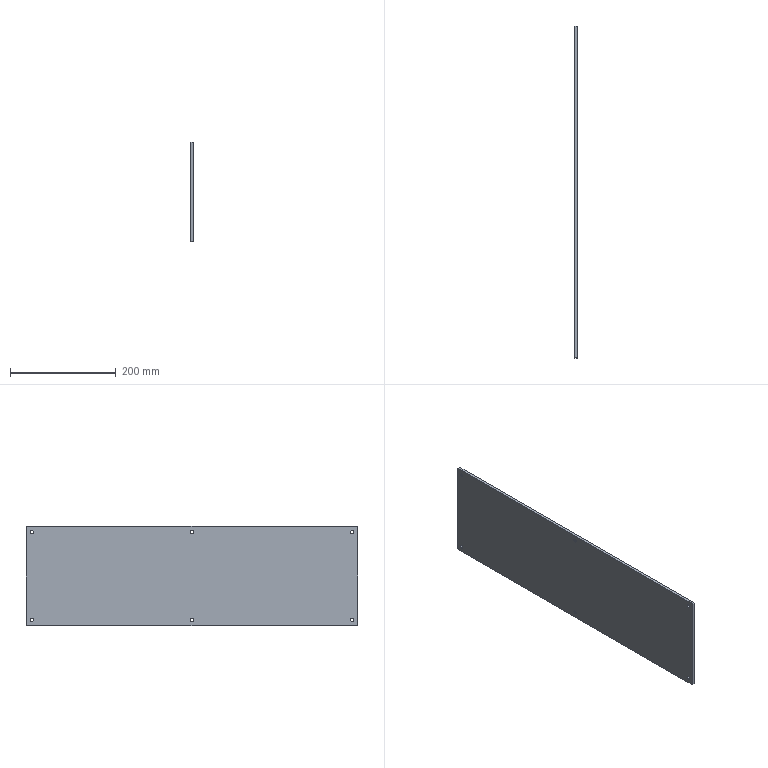Part | SolidWorks | features Chamfer 1, Extrusion 1, ICE 1 | 1 solid | 22 faces | box 5 x 628 x 188 mm | volume 589462 mm3 | cylinder 12 | plane 10 | commonest cylinder face diameters 6 x12
STEP:
#1=CARTESIAN_POINT('',(5.,0.,-86.));
#2=VERTEX_POINT('',#1);
#3=CARTESIAN_POINT('',(5.,0.,-80.));
#4=VERTEX_POINT('',#3);
#5=CARTESIAN_POINT('',(5.,0.,-83.));
#6=DIRECTION('',(-1.,0.,0.));
#7=DIRECTION('',(0.,0.,1.));
#8=AXIS2_PLACEMENT_3D('',#5,#6,#7);
#9=CIRCLE('',#8,3.);
#10=EDGE_CURVE('',#2,#4,#9,.T.);
#11=ORIENTED_EDGE('',*,*,#10,.F.);
#12=CARTESIAN_POINT('',(0.,0.,-86.));
#13=VERTEX_POINT('',#12);
#14=CARTESIAN_POINT('',(5.,0.,-86.));
#15=DIRECTION('',(-1.,0.,0.));
#16=VECTOR('',#15,1000.);
#17=LINE('',#14,#16);
#18=EDGE_CURVE('',#2,#13,#17,.T.);
#19=ORIENTED_EDGE('',*,*,#18,.T.);
#20=CARTESIAN_POINT('',(0.,0.,-80.));
#21=VERTEX_POINT('',#20);
#22=CARTESIAN_POINT('',(0.,0.,-83.));
#23=DIRECTION('',(-1.,0.,0.));
#24=DIRECTION('',(0.,0.,1.));
#25=AXIS2_PLACEMENT_3D('',#22,#23,#24);
#26=CIRCLE('',#25,3.);
#27=EDGE_CURVE('',#13,#21,#26,.T.);
#28=ORIENTED_EDGE('',*,*,#27,.T.);
#29=CARTESIAN_POINT('',(5.,0.,-80.));
#30=DIRECTION('',(-1.,0.,0.));
#31=VECTOR('',#30,1000.);
#32=LINE('',#29,#31);
#33=EDGE_CURVE('',#4,#21,#32,.T.);
#34=ORIENTED_EDGE('',*,*,#33,.F.);
#35=EDGE_LOOP('',(#11,#19,#28,#34));
#36=FACE_OUTER_BOUND('',#35,.T.);
#37=CARTESIAN_POINT('',(5.,0.,-83.));
#38=DIRECTION('',(-1.,0.,0.));
#39=DIRECTION('',(0.,0.,1.));
#40=AXIS2_PLACEMENT_3D('',#37,#38,#39);
#41=CYLINDRICAL_SURFACE('',#40,3.);
#42=ADVANCED_FACE('',(#36),#41,.F.);
#43=CARTESIAN_POINT('',(5.,0.,80.));
#44=VERTEX_POINT('',#43);
#45=CARTESIAN_POINT('',(5.,0.,86.));
#46=VERTEX_POINT('',#45);
#47=CARTESIAN_POINT('',(5.,0.,83.));
#48=DIRECTION('',(-1.,0.,0.));
#49=DIRECTION('',(0.,0.,1.));
#50=AXIS2_PLACEMENT_3D('',#47,#48,#49);
#51=CIRCLE('',#50,3.);
#52=EDGE_CURVE('',#44,#46,#51,.T.);
#53=ORIENTED_EDGE('',*,*,#52,.F.);
#54=CARTESIAN_POINT('',(0.,0.,80.));
#55=VERTEX_POINT('',#54);
#56=CARTESIAN_POINT('',(5.,0.,80.));
#57=DIRECTION('',(-1.,0.,0.));
#58=VECTOR('',#57,1000.);
#59=LINE('',#56,#58);
#60=EDGE_CURVE('',#44,#55,#59,.T.);
#61=ORIENTED_EDGE('',*,*,#60,.T.);
#62=CARTESIAN_POINT('',(0.,0.,86.));
#63=VERTEX_POINT('',#62);
#64=CARTESIAN_POINT('',(0.,0.,83.));
#65=DIRECTION('',(-1.,0.,0.));
#66=DIRECTION('',(0.,0.,1.));
#67=AXIS2_PLACEMENT_3D('',#64,#65,#66);
#68=CIRCLE('',#67,3.);
#69=EDGE_CURVE('',#55,#63,#68,.T.);
#70=ORIENTED_EDGE('',*,*,#69,.T.);
#71=CARTESIAN_POINT('',(5.,0.,86.));
#72=DIRECTION('',(-1.,0.,0.));
#73=VECTOR('',#72,1000.);
#74=LINE('',#71,#73);
#75=EDGE_CURVE('',#46,#63,#74,.T.);
#76=ORIENTED_EDGE('',*,*,#75,.F.);
#77=EDGE_LOOP('',(#53,#61,#70,#76));
#78=FACE_OUTER_BOUND('',#77,.T.);
#79=CARTESIAN_POINT('',(5.,0.,83.));
#80=DIRECTION('',(-1.,0.,0.));
#81=DIRECTION('',(0.,0.,1.));
#82=AXIS2_PLACEMENT_3D('',#79,#80,#81);
#83=CYLINDRICAL_SURFACE('',#82,3.);
#84=ADVANCED_FACE('',(#78),#83,.F.);
#85=CARTESIAN_POINT('',(5.,303.,80.));
#86=VERTEX_POINT('',#85);
#87=CARTESIAN_POINT('',(5.,303.,86.));
#88=VERTEX_POINT('',#87);
#89=CARTESIAN_POINT('',(5.,303.,83.));
#90=DIRECTION('',(-1.,0.,0.));
#91=DIRECTION('',(0.,0.,-1.));
#92=AXIS2_PLACEMENT_3D('',#89,#90,#91);
#93=CIRCLE('',#92,3.);
#94=EDGE_CURVE('',#86,#88,#93,.T.);
#95=ORIENTED_EDGE('',*,*,#94,.F.);
#96=CARTESIAN_POINT('',(0.,303.,80.));
#97=VERTEX_POINT('',#96);
#98=CARTESIAN_POINT('',(5.,303.,80.));
#99=DIRECTION('',(-1.,0.,0.));
#100=VECTOR('',#99,1000.);
#101=LINE('',#98,#100);
#102=EDGE_CURVE('',#86,#97,#101,.T.);
#103=ORIENTED_EDGE('',*,*,#102,.T.);
#104=CARTESIAN_POINT('',(0.,303.,86.));
#105=VERTEX_POINT('',#104);
#106=CARTESIAN_POINT('',(0.,303.,83.));
#107=DIRECTION('',(-1.,0.,0.));
#108=DIRECTION('',(0.,0.,-1.));
#109=AXIS2_PLACEMENT_3D('',#106,#107,#108);
#110=CIRCLE('',#109,3.);
#111=EDGE_CURVE('',#97,#105,#110,.T.);
#112=ORIENTED_EDGE('',*,*,#111,.T.);
#113=CARTESIAN_POINT('',(5.,303.,86.));
#114=DIRECTION('',(-1.,0.,0.));
#115=VECTOR('',#114,1000.);
#116=LINE('',#113,#115);
#117=EDGE_CURVE('',#88,#105,#116,.T.);
#118=ORIENTED_EDGE('',*,*,#117,.F.);
#119=EDGE_LOOP('',(#95,#103,#112,#118));
#120=FACE_OUTER_BOUND('',#119,.T.);
#121=CARTESIAN_POINT('',(5.,303.,83.));
#122=DIRECTION('',(-1.,0.,0.));
#123=DIRECTION('',(0.,0.,1.));
#124=AXIS2_PLACEMENT_3D('',#121,#122,#123);
#125=CYLINDRICAL_SURFACE('',#124,3.);
#126=ADVANCED_FACE('',(#120),#125,.F.);
#127=CARTESIAN_POINT('',(5.,-303.,80.));
#128=VERTEX_POINT('',#127);
#129=CARTESIAN_POINT('',(5.,-303.,86.));
#130=VERTEX_POINT('',#129);
#131=CARTESIAN_POINT('',(5.,-303.,83.));
#132=DIRECTION('',(-1.,0.,0.));
#133=DIRECTION('',(0.,0.,1.));
#134=AXIS2_PLACEMENT_3D('',#131,#132,#133);
#135=CIRCLE('',#134,3.);
#136=EDGE_CURVE('',#128,#130,#135,.T.);
#137=ORIENTED_EDGE('',*,*,#136,.F.);
#138=CARTESIAN_POINT('',(0.,-303.,80.));
#139=VERTEX_POINT('',#138);
#140=CARTESIAN_POINT('',(5.,-303.,80.));
#141=DIRECTION('',(-1.,0.,0.));
#142=VECTOR('',#141,1000.);
#143=LINE('',#140,#142);
#144=EDGE_CURVE('',#128,#139,#143,.T.);
#145=ORIENTED_EDGE('',*,*,#144,.T.);
#146=CARTESIAN_POINT('',(0.,-303.,86.));
#147=VERTEX_POINT('',#146);
#148=CARTESIAN_POINT('',(0.,-303.,83.));
#149=DIRECTION('',(-1.,0.,0.));
#150=DIRECTION('',(0.,0.,1.));
#151=AXIS2_PLACEMENT_3D('',#148,#149,#150);
#152=CIRCLE('',#151,3.);
#153=EDGE_CURVE('',#139,#147,#152,.T.);
#154=ORIENTED_EDGE('',*,*,#153,.T.);
#155=CARTESIAN_POINT('',(5.,-303.,86.));
#156=DIRECTION('',(-1.,0.,0.));
#157=VECTOR('',#156,1000.);
#158=LINE('',#155,#157);
#159=EDGE_CURVE('',#130,#147,#158,.T.);
#160=ORIENTED_EDGE('',*,*,#159,.F.);
#161=EDGE_LOOP('',(#137,#145,#154,#160));
#162=FACE_OUTER_BOUND('',#161,.T.);
#163=CARTESIAN_POINT('',(5.,-303.,83.));
#164=DIRECTION('',(-1.,0.,0.));
#165=DIRECTION('',(0.,0.,1.));
#166=AXIS2_PLACEMENT_3D('',#163,#164,#165);
#167=CYLINDRICAL_SURFACE('',#166,3.);
#168=ADVANCED_FACE('',(#162),#167,.F.);
#169=CARTESIAN_POINT('',(5.,-303.,-86.));
#170=VERTEX_POINT('',#169);
#171=CARTESIAN_POINT('',(5.,-303.,-80.));
#172=VERTEX_POINT('',#171);
#173=CARTESIAN_POINT('',(5.,-303.,-83.));
#174=DIRECTION('',(-1.,0.,0.));
#175=DIRECTION('',(0.,0.,-1.));
#176=AXIS2_PLACEMENT_3D('',#173,#174,#175);
#177=CIRCLE('',#176,3.);
#178=EDGE_CURVE('',#170,#172,#177,.T.);
#179=ORIENTED_EDGE('',*,*,#178,.F.);
#180=CARTESIAN_POINT('',(0.,-303.,-86.));
#181=VERTEX_POINT('',#180);
#182=CARTESIAN_POINT('',(5.,-303.,-86.));
#183=DIRECTION('',(-1.,0.,0.));
#184=VECTOR('',#183,1000.);
#185=LINE('',#182,#184);
#186=EDGE_CURVE('',#170,#181,#185,.T.);
#187=ORIENTED_EDGE('',*,*,#186,.T.);
#188=CARTESIAN_POINT('',(0.,-303.,-80.));
#189=VERTEX_POINT('',#188);
#190=CARTESIAN_POINT('',(0.,-303.,-83.));
#191=DIRECTION('',(-1.,0.,0.));
#192=DIRECTION('',(0.,0.,-1.));
#193=AXIS2_PLACEMENT_3D('',#190,#191,#192);
#194=CIRCLE('',#193,3.);
#195=EDGE_CURVE('',#181,#189,#194,.T.);
#196=ORIENTED_EDGE('',*,*,#195,.T.);
#197=CARTESIAN_POINT('',(5.,-303.,-80.));
#198=DIRECTION('',(-1.,0.,0.));
#199=VECTOR('',#198,1000.);
#200=LINE('',#197,#199);
#201=EDGE_CURVE('',#172,#189,#200,.T.);
#202=ORIENTED_EDGE('',*,*,#201,.F.);
#203=EDGE_LOOP('',(#179,#187,#196,#202));
#204=FACE_OUTER_BOUND('',#203,.T.);
#205=CARTESIAN_POINT('',(5.,-303.,-83.));
#206=DIRECTION('',(-1.,0.,0.));
#207=DIRECTION('',(0.,0.,1.));
#208=AXIS2_PLACEMENT_3D('',#205,#206,#207);
#209=CYLINDRICAL_SURFACE('',#208,3.);
#210=ADVANCED_FACE('',(#204),#209,.F.);
#211=CARTESIAN_POINT('',(5.,303.,-86.));
#212=VERTEX_POINT('',#211);
#213=CARTESIAN_POINT('',(5.,303.,-80.));
#214=VERTEX_POINT('',#213);
#215=CARTESIAN_POINT('',(5.,303.,-83.));
#216=DIRECTION('',(-1.,0.,0.));
#217=DIRECTION('',(0.,0.,1.));
#218=AXIS2_PLACEMENT_3D('',#215,#216,#217);
#219=CIRCLE('',#218,3.);
#220=EDGE_CURVE('',#212,#214,#219,.T.);
#221=ORIENTED_EDGE('',*,*,#220,.F.);
#222=CARTESIAN_POINT('',(0.,303.,-86.));
#223=VERTEX_POINT('',#222);
#224=CARTESIAN_POINT('',(5.,303.,-86.));
#225=DIRECTION('',(-1.,0.,0.));
#226=VECTOR('',#225,1000.);
#227=LINE('',#224,#226);
#228=EDGE_CURVE('',#212,#223,#227,.T.);
#229=ORIENTED_EDGE('',*,*,#228,.T.);
#230=CARTESIAN_POINT('',(0.,303.,-80.));
#231=VERTEX_POINT('',#230);
#232=CARTESIAN_POINT('',(0.,303.,-83.));
#233=DIRECTION('',(-1.,0.,0.));
#234=DIRECTION('',(0.,0.,1.));
#235=AXIS2_PLACEMENT_3D('',#232,#233,#234);
#236=CIRCLE('',#235,3.);
#237=EDGE_CURVE('',#223,#231,#236,.T.);
#238=ORIENTED_EDGE('',*,*,#237,.T.);
#239=CARTESIAN_POINT('',(5.,303.,-80.));
#240=DIRECTION('',(-1.,0.,0.));
#241=VECTOR('',#240,1000.);
#242=LINE('',#239,#241);
#243=EDGE_CURVE('',#214,#231,#242,.T.);
#244=ORIENTED_EDGE('',*,*,#243,.F.);
#245=EDGE_LOOP('',(#221,#229,#238,#244));
#246=FACE_OUTER_BOUND('',#245,.T.);
#247=CARTESIAN_POINT('',(5.,303.,-83.));
#248=DIRECTION('',(-1.,0.,0.));
#249=DIRECTION('',(0.,0.,1.));
#250=AXIS2_PLACEMENT_3D('',#247,#248,#249);
#251=CYLINDRICAL_SURFACE('',#250,3.);
#252=ADVANCED_FACE('',(#246),#251,.F.);
#253=CARTESIAN_POINT('',(0.,313.,94.));
#254=VERTEX_POINT('',#253);
#255=CARTESIAN_POINT('',(0.,-313.,94.));
#256=VERTEX_POINT('',#255);
#257=CARTESIAN_POINT('',(0.,314.,94.));
#258=DIRECTION('',(0.,-1.,0.));
#259=VECTOR('',#258,1000.);
#260=LINE('',#257,#259);
#261=EDGE_CURVE('',#254,#256,#260,.T.);
#262=ORIENTED_EDGE('',*,*,#261,.T.);
#263=CARTESIAN_POINT('',(5.,-313.,94.));
#264=VERTEX_POINT('',#263);
#265=CARTESIAN_POINT('',(5.,-313.,94.));
#266=DIRECTION('',(1.,0.,0.));
#267=VECTOR('',#266,1000.);
#268=LINE('',#265,#267);
#269=EDGE_CURVE('',#256,#264,#268,.T.);
#270=ORIENTED_EDGE('',*,*,#269,.T.);
#271=CARTESIAN_POINT('',(5.,313.,94.));
#272=VERTEX_POINT('',#271);
#273=CARTESIAN_POINT('',(5.,314.,94.));
#274=DIRECTION('',(0.,-1.,0.));
#275=VECTOR('',#274,1000.);
#276=LINE('',#273,#275);
#277=EDGE_CURVE('',#272,#264,#276,.T.);
#278=ORIENTED_EDGE('',*,*,#277,.F.);
#279=CARTESIAN_POINT('',(5.,313.,94.));
#280=DIRECTION('',(-1.,0.,0.));
#281=VECTOR('',#280,1000.);
#282=LINE('',#279,#281);
#283=EDGE_CURVE('',#272,#254,#282,.T.);
#284=ORIENTED_EDGE('',*,*,#283,.T.);
#285=EDGE_LOOP('',(#262,#270,#278,#284));
#286=FACE_OUTER_BOUND('',#285,.T.);
#287=CARTESIAN_POINT('',(5.,314.,94.));
#288=DIRECTION('',(0.,0.,-1.));
#289=DIRECTION('',(0.,1.,0.));
#290=AXIS2_PLACEMENT_3D('',#287,#288,#289);
#291=PLANE('',#290);
#292=ADVANCED_FACE('',(#286),#291,.F.);
#293=CARTESIAN_POINT('',(0.,-314.,93.));
#294=VERTEX_POINT('',#293);
#295=CARTESIAN_POINT('',(0.,-314.,-93.));
#296=VERTEX_POINT('',#295);
#297=CARTESIAN_POINT('',(0.,-314.,-94.));
#298=DIRECTION('',(0.,0.,-1.));
#299=VECTOR('',#298,1000.);
#300=LINE('',#297,#299);
#301=EDGE_CURVE('',#294,#296,#300,.T.);
#302=ORIENTED_EDGE('',*,*,#301,.T.);
#303=CARTESIAN_POINT('',(5.,-314.,-93.));
#304=VERTEX_POINT('',#303);
#305=CARTESIAN_POINT('',(5.,-314.,-93.));
#306=DIRECTION('',(1.,0.,0.));
#307=VECTOR('',#306,1000.);
#308=LINE('',#305,#307);
#309=EDGE_CURVE('',#296,#304,#308,.T.);
#310=ORIENTED_EDGE('',*,*,#309,.T.);
#311=CARTESIAN_POINT('',(5.,-314.,93.));
#312=VERTEX_POINT('',#311);
#313=CARTESIAN_POINT('',(5.,-314.,-94.));
#314=DIRECTION('',(0.,0.,-1.));
#315=VECTOR('',#314,1000.);
#316=LINE('',#313,#315);
#317=EDGE_CURVE('',#312,#304,#316,.T.);
#318=ORIENTED_EDGE('',*,*,#317,.F.);
#319=CARTESIAN_POINT('',(5.,-314.,93.));
#320=DIRECTION('',(-1.,0.,0.));
#321=VECTOR('',#320,1000.);
#322=LINE('',#319,#321);
#323=EDGE_CURVE('',#312,#294,#322,.T.);
#324=ORIENTED_EDGE('',*,*,#323,.T.);
#325=EDGE_LOOP('',(#302,#310,#318,#324));
#326=FACE_OUTER_BOUND('',#325,.T.);
#327=CARTESIAN_POINT('',(5.,-314.,-94.));
#328=DIRECTION('',(0.,1.,0.));
#329=DIRECTION('',(0.,0.,1.));
#330=AXIS2_PLACEMENT_3D('',#327,#328,#329);
#331=PLANE('',#330);
#332=ADVANCED_FACE('',(#326),#331,.F.);
#333=CARTESIAN_POINT('',(5.,-313.,-94.));
#334=VERTEX_POINT('',#333);
#335=CARTESIAN_POINT('',(5.,313.,-94.));
#336=VERTEX_POINT('',#335);
#337=CARTESIAN_POINT('',(5.,314.,-94.));
#338=DIRECTION('',(0.,1.,0.));
#339=VECTOR('',#338,1000.);
#340=LINE('',#337,#339);
#341=EDGE_CURVE('',#334,#336,#340,.T.);
#342=ORIENTED_EDGE('',*,*,#341,.F.);
#343=CARTESIAN_POINT('',(0.,-313.,-94.));
#344=VERTEX_POINT('',#343);
#345=CARTESIAN_POINT('',(5.,-313.,-94.));
#346=DIRECTION('',(-1.,0.,0.));
#347=VECTOR('',#346,1000.);
#348=LINE('',#345,#347);
#349=EDGE_CURVE('',#334,#344,#348,.T.);
#350=ORIENTED_EDGE('',*,*,#349,.T.);
#351=CARTESIAN_POINT('',(0.,313.,-94.));
#352=VERTEX_POINT('',#351);
#353=CARTESIAN_POINT('',(0.,314.,-94.));
#354=DIRECTION('',(0.,1.,0.));
#355=VECTOR('',#354,1000.);
#356=LINE('',#353,#355);
#357=EDGE_CURVE('',#344,#352,#356,.T.);
#358=ORIENTED_EDGE('',*,*,#357,.T.);
#359=CARTESIAN_POINT('',(5.,313.,-94.));
#360=DIRECTION('',(1.,0.,0.));
#361=VECTOR('',#360,1000.);
#362=LINE('',#359,#361);
#363=EDGE_CURVE('',#352,#336,#362,.T.);
#364=ORIENTED_EDGE('',*,*,#363,.T.);
#365=EDGE_LOOP('',(#342,#350,#358,#364));
#366=FACE_OUTER_BOUND('',#365,.T.);
#367=CARTESIAN_POINT('',(5.,314.,-94.));
#368=DIRECTION('',(0.,0.,1.));
#369=DIRECTION('',(0.,-1.,0.));
#370=AXIS2_PLACEMENT_3D('',#367,#368,#369);
#371=PLANE('',#370);
#372=ADVANCED_FACE('',(#366),#371,.F.);
#373=CARTESIAN_POINT('',(5.,314.,-93.));
#374=VERTEX_POINT('',#373);
#375=CARTESIAN_POINT('',(5.,314.,93.));
#376=VERTEX_POINT('',#375);
#377=CARTESIAN_POINT('',(5.,314.,-94.));
#378=DIRECTION('',(0.,0.,1.));
#379=VECTOR('',#378,1000.);
#380=LINE('',#377,#379);
#381=EDGE_CURVE('',#374,#376,#380,.T.);
#382=ORIENTED_EDGE('',*,*,#381,.F.);
#383=CARTESIAN_POINT('',(0.,314.,-93.));
#384=VERTEX_POINT('',#383);
#385=CARTESIAN_POINT('',(5.,314.,-93.));
#386=DIRECTION('',(-1.,0.,0.));
#387=VECTOR('',#386,1000.);
#388=LINE('',#385,#387);
#389=EDGE_CURVE('',#374,#384,#388,.T.);
#390=ORIENTED_EDGE('',*,*,#389,.T.);
#391=CARTESIAN_POINT('',(0.,314.,93.));
#392=VERTEX_POINT('',#391);
#393=CARTESIAN_POINT('',(0.,314.,-94.));
#394=DIRECTION('',(0.,0.,1.));
#395=VECTOR('',#394,1000.);
#396=LINE('',#393,#395);
#397=EDGE_CURVE('',#384,#392,#396,.T.);
#398=ORIENTED_EDGE('',*,*,#397,.T.);
#399=CARTESIAN_POINT('',(5.,314.,93.));
#400=DIRECTION('',(1.,0.,0.));
#401=VECTOR('',#400,1000.);
#402=LINE('',#399,#401);
#403=EDGE_CURVE('',#392,#376,#402,.T.);
#404=ORIENTED_EDGE('',*,*,#403,.T.);
#405=EDGE_LOOP('',(#382,#390,#398,#404));
#406=FACE_OUTER_BOUND('',#405,.T.);
#407=CARTESIAN_POINT('',(5.,314.,-94.));
#408=DIRECTION('',(0.,-1.,0.));
#409=DIRECTION('',(0.,0.,-1.));
#410=AXIS2_PLACEMENT_3D('',#407,#408,#409);
#411=PLANE('',#410);
#412=ADVANCED_FACE('',(#406),#411,.F.);
#413=CARTESIAN_POINT('',(5.,0.,-83.));
#414=DIRECTION('',(-1.,0.,0.));
#415=DIRECTION('',(0.,0.,1.));
#416=AXIS2_PLACEMENT_3D('',#413,#414,#415);
#417=CIRCLE('',#416,3.);
#418=EDGE_CURVE('',#4,#2,#417,.T.);
#419=ORIENTED_EDGE('',*,*,#418,.T.);
#420=ORIENTED_EDGE('',*,*,#10,.T.);
#421=EDGE_LOOP('',(#419,#420));
#422=FACE_BOUND('',#421,.T.);
#423=CARTESIAN_POINT('',(5.,0.,83.));
#424=DIRECTION('',(-1.,0.,0.));
#425=DIRECTION('',(0.,0.,1.));
#426=AXIS2_PLACEMENT_3D('',#423,#424,#425);
#427=CIRCLE('',#426,3.);
#428=EDGE_CURVE('',#46,#44,#427,.T.);
#429=ORIENTED_EDGE('',*,*,#428,.T.);
#430=ORIENTED_EDGE('',*,*,#52,.T.);
#431=EDGE_LOOP('',(#429,#430));
#432=FACE_BOUND('',#431,.T.);
#433=CARTESIAN_POINT('',(5.,303.,83.));
#434=DIRECTION('',(-1.,0.,0.));
#435=DIRECTION('',(0.,0.,-1.));
#436=AXIS2_PLACEMENT_3D('',#433,#434,#435);
#437=CIRCLE('',#436,3.);
#438=EDGE_CURVE('',#88,#86,#437,.T.);
#439=ORIENTED_EDGE('',*,*,#438,.T.);
#440=ORIENTED_EDGE('',*,*,#94,.T.);
#441=EDGE_LOOP('',(#439,#440));
#442=FACE_BOUND('',#441,.T.);
#443=CARTESIAN_POINT('',(5.,-303.,83.));
#444=DIRECTION('',(-1.,0.,0.));
#445=DIRECTION('',(0.,0.,1.));
#446=AXIS2_PLACEMENT_3D('',#443,#444,#445);
#447=CIRCLE('',#446,3.);
#448=EDGE_CURVE('',#130,#128,#447,.T.);
#449=ORIENTED_EDGE('',*,*,#448,.T.);
#450=ORIENTED_EDGE('',*,*,#136,.T.);
#451=EDGE_LOOP('',(#449,#450));
#452=FACE_BOUND('',#451,.T.);
#453=CARTESIAN_POINT('',(5.,-303.,-83.));
#454=DIRECTION('',(-1.,0.,0.));
#455=DIRECTION('',(0.,0.,-1.));
#456=AXIS2_PLACEMENT_3D('',#453,#454,#455);
#457=CIRCLE('',#456,3.);
#458=EDGE_CURVE('',#172,#170,#457,.T.);
#459=ORIENTED_EDGE('',*,*,#458,.T.);
#460=ORIENTED_EDGE('',*,*,#178,.T.);
#461=EDGE_LOOP('',(#459,#460));
#462=FACE_BOUND('',#461,.T.);
#463=CARTESIAN_POINT('',(5.,303.,-83.));
#464=DIRECTION('',(-1.,0.,0.));
#465=DIRECTION('',(0.,0.,1.));
#466=AXIS2_PLACEMENT_3D('',#463,#464,#465);
#467=CIRCLE('',#466,3.);
#468=EDGE_CURVE('',#214,#212,#467,.T.);
#469=ORIENTED_EDGE('',*,*,#468,.T.);
#470=ORIENTED_EDGE('',*,*,#220,.T.);
#471=EDGE_LOOP('',(#469,#470));
#472=FACE_BOUND('',#471,.T.);
#473=ORIENTED_EDGE('',*,*,#317,.T.);
#474=CARTESIAN_POINT('',(5.,-313.,-94.));
#475=DIRECTION('',(0.,0.7071,-0.7071));
#476=VECTOR('',#475,1000.);
#477=LINE('',#474,#476);
#478=EDGE_CURVE('',#304,#334,#477,.T.);
#479=ORIENTED_EDGE('',*,*,#478,.T.);
#480=ORIENTED_EDGE('',*,*,#341,.T.);
#481=CARTESIAN_POINT('',(5.,314.,-93.));
#482=DIRECTION('',(0.,0.7071,0.7071));
#483=VECTOR('',#482,1000.);
#484=LINE('',#481,#483);
#485=EDGE_CURVE('',#336,#374,#484,.T.);
#486=ORIENTED_EDGE('',*,*,#485,.T.);
#487=ORIENTED_EDGE('',*,*,#381,.T.);
#488=CARTESIAN_POINT('',(5.,313.,94.));
#489=DIRECTION('',(0.,-0.7071,0.7071));
#490=VECTOR('',#489,1000.);
#491=LINE('',#488,#490);
#492=EDGE_CURVE('',#376,#272,#491,.T.);
#493=ORIENTED_EDGE('',*,*,#492,.T.);
#494=ORIENTED_EDGE('',*,*,#277,.T.);
#495=CARTESIAN_POINT('',(5.,-314.,93.));
#496=DIRECTION('',(0.,-0.7071,-0.7071));
#497=VECTOR('',#496,1000.);
#498=LINE('',#495,#497);
#499=EDGE_CURVE('',#264,#312,#498,.T.);
#500=ORIENTED_EDGE('',*,*,#499,.T.);
#501=EDGE_LOOP('',(#473,#479,#480,#486,#487,#493,#494,#500));
#502=FACE_OUTER_BOUND('',#501,.T.);
#503=CARTESIAN_POINT('',(5.,-314.,94.));
#504=DIRECTION('',(-1.,0.,0.));
#505=DIRECTION('',(0.,0.,1.));
#506=AXIS2_PLACEMENT_3D('',#503,#504,#505);
#507=PLANE('',#506);
#508=ADVANCED_FACE('',(#422,#432,#442,#452,#462,#472,#502),#507,.F.);
#509=CARTESIAN_POINT('',(0.,0.,-83.));
#510=DIRECTION('',(-1.,0.,0.));
#511=DIRECTION('',(0.,0.,1.));
#512=AXIS2_PLACEMENT_3D('',#509,#510,#511);
#513=CIRCLE('',#512,3.);
#514=EDGE_CURVE('',#21,#13,#513,.T.);
#515=ORIENTED_EDGE('',*,*,#514,.F.);
#516=ORIENTED_EDGE('',*,*,#27,.F.);
#517=EDGE_LOOP('',(#515,#516));
#518=FACE_BOUND('',#517,.T.);
#519=CARTESIAN_POINT('',(0.,0.,83.));
#520=DIRECTION('',(-1.,0.,0.));
#521=DIRECTION('',(0.,0.,1.));
#522=AXIS2_PLACEMENT_3D('',#519,#520,#521);
#523=CIRCLE('',#522,3.);
#524=EDGE_CURVE('',#63,#55,#523,.T.);
#525=ORIENTED_EDGE('',*,*,#524,.F.);
#526=ORIENTED_EDGE('',*,*,#69,.F.);
#527=EDGE_LOOP('',(#525,#526));
#528=FACE_BOUND('',#527,.T.);
#529=CARTESIAN_POINT('',(0.,303.,83.));
#530=DIRECTION('',(-1.,0.,0.));
#531=DIRECTION('',(0.,0.,-1.));
#532=AXIS2_PLACEMENT_3D('',#529,#530,#531);
#533=CIRCLE('',#532,3.);
#534=EDGE_CURVE('',#105,#97,#533,.T.);
#535=ORIENTED_EDGE('',*,*,#534,.F.);
#536=ORIENTED_EDGE('',*,*,#111,.F.);
#537=EDGE_LOOP('',(#535,#536));
#538=FACE_BOUND('',#537,.T.);
#539=CARTESIAN_POINT('',(0.,-303.,83.));
#540=DIRECTION('',(-1.,0.,0.));
#541=DIRECTION('',(0.,0.,1.));
#542=AXIS2_PLACEMENT_3D('',#539,#540,#541);
#543=CIRCLE('',#542,3.);
#544=EDGE_CURVE('',#147,#139,#543,.T.);
#545=ORIENTED_EDGE('',*,*,#544,.F.);
#546=ORIENTED_EDGE('',*,*,#153,.F.);
#547=EDGE_LOOP('',(#545,#546));
#548=FACE_BOUND('',#547,.T.);
#549=CARTESIAN_POINT('',(0.,-303.,-83.));
#550=DIRECTION('',(-1.,0.,0.));
#551=DIRECTION('',(0.,0.,-1.));
#552=AXIS2_PLACEMENT_3D('',#549,#550,#551);
#553=CIRCLE('',#552,3.);
#554=EDGE_CURVE('',#189,#181,#553,.T.);
#555=ORIENTED_EDGE('',*,*,#554,.F.);
#556=ORIENTED_EDGE('',*,*,#195,.F.);
#557=EDGE_LOOP('',(#555,#556));
#558=FACE_BOUND('',#557,.T.);
#559=CARTESIAN_POINT('',(0.,303.,-83.));
#560=DIRECTION('',(-1.,0.,0.));
#561=DIRECTION('',(0.,0.,1.));
#562=AXIS2_PLACEMENT_3D('',#559,#560,#561);
#563=CIRCLE('',#562,3.);
#564=EDGE_CURVE('',#231,#223,#563,.T.);
#565=ORIENTED_EDGE('',*,*,#564,.F.);
#566=ORIENTED_EDGE('',*,*,#237,.F.);
#567=EDGE_LOOP('',(#565,#566));
#568=FACE_BOUND('',#567,.T.);
#569=ORIENTED_EDGE('',*,*,#357,.F.);
#570=CARTESIAN_POINT('',(0.,-407.5,0.5));
#571=DIRECTION('',(0.,-0.7071,0.7071));
#572=VECTOR('',#571,1000.);
#573=LINE('',#570,#572);
#574=EDGE_CURVE('',#344,#296,#573,.T.);
#575=ORIENTED_EDGE('',*,*,#574,.T.);
#576=ORIENTED_EDGE('',*,*,#301,.F.);
#577=CARTESIAN_POINT('',(0.,-313.5,93.5));
#578=DIRECTION('',(0.,0.7071,0.7071));
#579=VECTOR('',#578,1000.);
#580=LINE('',#577,#579);
#581=EDGE_CURVE('',#294,#256,#580,.T.);
#582=ORIENTED_EDGE('',*,*,#581,.T.);
#583=ORIENTED_EDGE('',*,*,#261,.F.);
#584=CARTESIAN_POINT('',(0.,-0.5,407.5));
#585=DIRECTION('',(0.,0.7071,-0.7071));
#586=VECTOR('',#585,1000.);
#587=LINE('',#584,#586);
#588=EDGE_CURVE('',#254,#392,#587,.T.);
#589=ORIENTED_EDGE('',*,*,#588,.T.);
#590=ORIENTED_EDGE('',*,*,#397,.F.);
#591=CARTESIAN_POINT('',(0.,93.5,-313.5));
#592=DIRECTION('',(0.,-0.7071,-0.7071));
#593=VECTOR('',#592,1000.);
#594=LINE('',#591,#593);
#595=EDGE_CURVE('',#384,#352,#594,.T.);
#596=ORIENTED_EDGE('',*,*,#595,.T.);
#597=EDGE_LOOP('',(#569,#575,#576,#582,#583,#589,#590,#596));
#598=FACE_OUTER_BOUND('',#597,.T.);
#599=CARTESIAN_POINT('',(0.,-314.,94.));
#600=DIRECTION('',(-1.,0.,0.));
#601=DIRECTION('',(0.,0.,1.));
#602=AXIS2_PLACEMENT_3D('',#599,#600,#601);
#603=PLANE('',#602);
#604=ADVANCED_FACE('',(#518,#528,#538,#548,#558,#568,#598),#603,.T.);
#605=ORIENTED_EDGE('',*,*,#478,.F.);
#606=ORIENTED_EDGE('',*,*,#309,.F.);
#607=ORIENTED_EDGE('',*,*,#574,.F.);
#608=ORIENTED_EDGE('',*,*,#349,.F.);
#609=EDGE_LOOP('',(#605,#606,#607,#608));
#610=FACE_OUTER_BOUND('',#609,.T.);
#611=CARTESIAN_POINT('',(5.,-313.,-94.));
#612=DIRECTION('',(0.,0.7071,0.7071));
#613=DIRECTION('',(0.,-0.7071,0.7071));
#614=AXIS2_PLACEMENT_3D('',#611,#612,#613);
#615=PLANE('',#614);
#616=ADVANCED_FACE('',(#610),#615,.F.);
#617=ORIENTED_EDGE('',*,*,#499,.F.);
#618=ORIENTED_EDGE('',*,*,#269,.F.);
#619=ORIENTED_EDGE('',*,*,#581,.F.);
#620=ORIENTED_EDGE('',*,*,#323,.F.);
#621=EDGE_LOOP('',(#617,#618,#619,#620));
#622=FACE_OUTER_BOUND('',#621,.T.);
#623=CARTESIAN_POINT('',(5.,-314.,93.));
#624=DIRECTION('',(0.,0.7071,-0.7071));
#625=DIRECTION('',(0.,0.7071,0.7071));
#626=AXIS2_PLACEMENT_3D('',#623,#624,#625);
#627=PLANE('',#626);
#628=ADVANCED_FACE('',(#622),#627,.F.);
#629=ORIENTED_EDGE('',*,*,#485,.F.);
#630=ORIENTED_EDGE('',*,*,#363,.F.);
#631=ORIENTED_EDGE('',*,*,#595,.F.);
#632=ORIENTED_EDGE('',*,*,#389,.F.);
#633=EDGE_LOOP('',(#629,#630,#631,#632));
#634=FACE_OUTER_BOUND('',#633,.T.);
#635=CARTESIAN_POINT('',(5.,314.,-93.));
#636=DIRECTION('',(0.,-0.7071,0.7071));
#637=DIRECTION('',(0.,-0.7071,-0.7071));
#638=AXIS2_PLACEMENT_3D('',#635,#636,#637);
#639=PLANE('',#638);
#640=ADVANCED_FACE('',(#634),#639,.F.);
#641=ORIENTED_EDGE('',*,*,#492,.F.);
#642=ORIENTED_EDGE('',*,*,#403,.F.);
#643=ORIENTED_EDGE('',*,*,#588,.F.);
#644=ORIENTED_EDGE('',*,*,#283,.F.);
#645=EDGE_LOOP('',(#641,#642,#643,#644));
#646=FACE_OUTER_BOUND('',#645,.T.);
#647=CARTESIAN_POINT('',(5.,313.,94.));
#648=DIRECTION('',(0.,-0.7071,-0.7071));
#649=DIRECTION('',(0.,0.7071,-0.7071));
#650=AXIS2_PLACEMENT_3D('',#647,#648,#649);
#651=PLANE('',#650);
#652=ADVANCED_FACE('',(#646),#651,.F.);
#653=ORIENTED_EDGE('',*,*,#228,.F.);
#654=ORIENTED_EDGE('',*,*,#468,.F.);
#655=ORIENTED_EDGE('',*,*,#243,.T.);
#656=ORIENTED_EDGE('',*,*,#564,.T.);
#657=EDGE_LOOP('',(#653,#654,#655,#656));
#658=FACE_OUTER_BOUND('',#657,.T.);
#659=CARTESIAN_POINT('',(5.,303.,-83.));
#660=DIRECTION('',(-1.,0.,0.));
#661=DIRECTION('',(0.,0.,1.));
#662=AXIS2_PLACEMENT_3D('',#659,#660,#661);
#663=CYLINDRICAL_SURFACE('',#662,3.);
#664=ADVANCED_FACE('',(#658),#663,.F.);
#665=ORIENTED_EDGE('',*,*,#186,.F.);
#666=ORIENTED_EDGE('',*,*,#458,.F.);
#667=ORIENTED_EDGE('',*,*,#201,.T.);
#668=ORIENTED_EDGE('',*,*,#554,.T.);
#669=EDGE_LOOP('',(#665,#666,#667,#668));
#670=FACE_OUTER_BOUND('',#669,.T.);
#671=CARTESIAN_POINT('',(5.,-303.,-83.));
#672=DIRECTION('',(-1.,0.,0.));
#673=DIRECTION('',(0.,0.,1.));
#674=AXIS2_PLACEMENT_3D('',#671,#672,#673);
#675=CYLINDRICAL_SURFACE('',#674,3.);
#676=ADVANCED_FACE('',(#670),#675,.F.);
#677=ORIENTED_EDGE('',*,*,#144,.F.);
#678=ORIENTED_EDGE('',*,*,#448,.F.);
#679=ORIENTED_EDGE('',*,*,#159,.T.);
#680=ORIENTED_EDGE('',*,*,#544,.T.);
#681=EDGE_LOOP('',(#677,#678,#679,#680));
#682=FACE_OUTER_BOUND('',#681,.T.);
#683=CARTESIAN_POINT('',(5.,-303.,83.));
#684=DIRECTION('',(-1.,0.,0.));
#685=DIRECTION('',(0.,0.,1.));
#686=AXIS2_PLACEMENT_3D('',#683,#684,#685);
#687=CYLINDRICAL_SURFACE('',#686,3.);
#688=ADVANCED_FACE('',(#682),#687,.F.);
#689=ORIENTED_EDGE('',*,*,#102,.F.);
#690=ORIENTED_EDGE('',*,*,#438,.F.);
#691=ORIENTED_EDGE('',*,*,#117,.T.);
#692=ORIENTED_EDGE('',*,*,#534,.T.);
#693=EDGE_LOOP('',(#689,#690,#691,#692));
#694=FACE_OUTER_BOUND('',#693,.T.);
#695=CARTESIAN_POINT('',(5.,303.,83.));
#696=DIRECTION('',(-1.,0.,0.));
#697=DIRECTION('',(0.,0.,1.));
#698=AXIS2_PLACEMENT_3D('',#695,#696,#697);
#699=CYLINDRICAL_SURFACE('',#698,3.);
#700=ADVANCED_FACE('',(#694),#699,.F.);
#701=ORIENTED_EDGE('',*,*,#60,.F.);
#702=ORIENTED_EDGE('',*,*,#428,.F.);
#703=ORIENTED_EDGE('',*,*,#75,.T.);
#704=ORIENTED_EDGE('',*,*,#524,.T.);
#705=EDGE_LOOP('',(#701,#702,#703,#704));
#706=FACE_OUTER_BOUND('',#705,.T.);
#707=CARTESIAN_POINT('',(5.,0.,83.));
#708=DIRECTION('',(-1.,0.,0.));
#709=DIRECTION('',(0.,0.,1.));
#710=AXIS2_PLACEMENT_3D('',#707,#708,#709);
#711=CYLINDRICAL_SURFACE('',#710,3.);
#712=ADVANCED_FACE('',(#706),#711,.F.);
#713=ORIENTED_EDGE('',*,*,#18,.F.);
#714=ORIENTED_EDGE('',*,*,#418,.F.);
#715=ORIENTED_EDGE('',*,*,#33,.T.);
#716=ORIENTED_EDGE('',*,*,#514,.T.);
#717=EDGE_LOOP('',(#713,#714,#715,#716));
#718=FACE_OUTER_BOUND('',#717,.T.);
#719=CARTESIAN_POINT('',(5.,0.,-83.));
#720=DIRECTION('',(-1.,0.,0.));
#721=DIRECTION('',(0.,0.,1.));
#722=AXIS2_PLACEMENT_3D('',#719,#720,#721);
#723=CYLINDRICAL_SURFACE('',#722,3.);
#724=ADVANCED_FACE('',(#718),#723,.F.);
#725=CLOSED_SHELL('',(#42,#84,#126,#168,#210,#252,#292,#332,#372,#412,#508,#604,#616,#628,#640,#652,#664,#676,#688,#700,#712,#724));
#726=MANIFOLD_SOLID_BREP('',#725);
#727=CARTESIAN_POINT('',(0.,0.,0.));
#728=DIRECTION('',(0.,0.,1.));
#729=DIRECTION('',(1.,0.,0.));
#730=AXIS2_PLACEMENT_3D('',#727,#728,#729);
#731=(LENGTH_UNIT()NAMED_UNIT(*)SI_UNIT(.MILLI.,.METRE.));
#732=UNCERTAINTY_MEASURE_WITH_UNIT(LENGTH_MEASURE(0.00001),#731,'','');
#733=(NAMED_UNIT(*)PLANE_ANGLE_UNIT()SI_UNIT($,.RADIAN.));
#734=(NAMED_UNIT(*)SI_UNIT($,.STERADIAN.)SOLID_ANGLE_UNIT());
#735=(GEOMETRIC_REPRESENTATION_CONTEXT(3)GLOBAL_UNCERTAINTY_ASSIGNED_CONTEXT((#732))GLOBAL_UNIT_ASSIGNED_CONTEXT((#731,#733,#734))REPRESENTATION_CONTEXT('',''));
#736=ADVANCED_BREP_SHAPE_REPRESENTATION('',(#726,#730),#735);